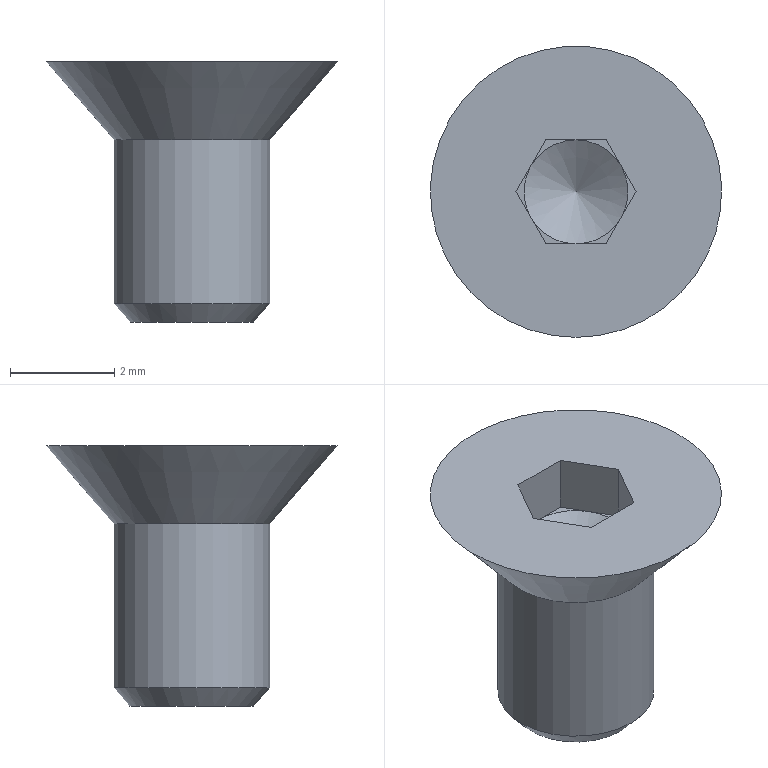Part | NX | features 5003_325_C-SFB3-5 2 | 1 solid | 18 faces | box 5.6 x 5.6 x 5 mm | volume 42.271 mm3 | plane 14 | cone 3 | cylinder 1 | commonest cylinder face diameters 3 x1
STEP:
#1=CARTESIAN_POINT('',(256.67,-34.6,-19.5));
#2=VERTEX_POINT('',#1);
#3=CARTESIAN_POINT('',(257.248,-35.6,-19.5));
#4=VERTEX_POINT('',#3);
#5=CARTESIAN_POINT('',(256.67,-34.6,-19.5));
#6=DIRECTION('',(0.5,-0.866,0.));
#7=VECTOR('',#6,1000.);
#8=LINE('',#5,#7);
#9=EDGE_CURVE('',#2,#4,#8,.T.);
#10=ORIENTED_EDGE('',*,*,#9,.F.);
#11=CARTESIAN_POINT('',(257.248,-33.6,-19.5));
#12=VERTEX_POINT('',#11);
#13=CARTESIAN_POINT('',(257.248,-33.6,-19.5));
#14=DIRECTION('',(-0.5,-0.866,0.));
#15=VECTOR('',#14,1000.);
#16=LINE('',#13,#15);
#17=EDGE_CURVE('',#12,#2,#16,.T.);
#18=ORIENTED_EDGE('',*,*,#17,.F.);
#19=CARTESIAN_POINT('',(258.402,-33.6,-19.5));
#20=VERTEX_POINT('',#19);
#21=CARTESIAN_POINT('',(258.402,-33.6,-19.5));
#22=DIRECTION('',(-1.,0.,0.));
#23=VECTOR('',#22,1000.);
#24=LINE('',#21,#23);
#25=EDGE_CURVE('',#20,#12,#24,.T.);
#26=ORIENTED_EDGE('',*,*,#25,.F.);
#27=CARTESIAN_POINT('',(258.98,-34.6,-19.5));
#28=VERTEX_POINT('',#27);
#29=CARTESIAN_POINT('',(258.98,-34.6,-19.5));
#30=DIRECTION('',(-0.5,0.866,0.));
#31=VECTOR('',#30,1000.);
#32=LINE('',#29,#31);
#33=EDGE_CURVE('',#28,#20,#32,.T.);
#34=ORIENTED_EDGE('',*,*,#33,.F.);
#35=CARTESIAN_POINT('',(258.402,-35.6,-19.5));
#36=VERTEX_POINT('',#35);
#37=CARTESIAN_POINT('',(258.402,-35.6,-19.5));
#38=DIRECTION('',(0.5,0.866,0.));
#39=VECTOR('',#38,1000.);
#40=LINE('',#37,#39);
#41=EDGE_CURVE('',#36,#28,#40,.T.);
#42=ORIENTED_EDGE('',*,*,#41,.F.);
#43=CARTESIAN_POINT('',(257.248,-35.6,-19.5));
#44=DIRECTION('',(1.,0.,0.));
#45=VECTOR('',#44,1000.);
#46=LINE('',#43,#45);
#47=EDGE_CURVE('',#4,#36,#46,.T.);
#48=ORIENTED_EDGE('',*,*,#47,.F.);
#49=EDGE_LOOP('',(#10,#18,#26,#34,#42,#48));
#50=FACE_BOUND('',#49,.T.);
#51=CARTESIAN_POINT('',(257.825,-37.4,-19.5));
#52=VERTEX_POINT('',#51);
#53=CARTESIAN_POINT('',(257.825,-34.6,-19.5));
#54=DIRECTION('',(0.,0.,-1.));
#55=DIRECTION('',(0.,-1.,0.));
#56=AXIS2_PLACEMENT_3D('',#53,#54,#55);
#57=CIRCLE('',#56,2.8);
#58=EDGE_CURVE('',#52,#52,#57,.T.);
#59=ORIENTED_EDGE('',*,*,#58,.F.);
#60=EDGE_LOOP('',(#59));
#61=FACE_BOUND('',#60,.T.);
#62=CARTESIAN_POINT('',(257.825,-34.6,-19.5));
#63=DIRECTION('',(0.,0.,1.));
#64=DIRECTION('',(0.,1.,0.));
#65=AXIS2_PLACEMENT_3D('',#62,#63,#64);
#66=PLANE('',#65);
#67=ADVANCED_FACE('',(#50,#61),#66,.T.);
#68=ORIENTED_EDGE('',*,*,#58,.T.);
#69=EDGE_LOOP('',(#68));
#70=FACE_BOUND('',#69,.T.);
#71=CARTESIAN_POINT('',(257.825,-36.1,-21.));
#72=VERTEX_POINT('',#71);
#73=CARTESIAN_POINT('',(257.825,-34.6,-21.));
#74=DIRECTION('',(0.,0.,-1.));
#75=DIRECTION('',(0.,-1.,0.));
#76=AXIS2_PLACEMENT_3D('',#73,#74,#75);
#77=CIRCLE('',#76,1.5);
#78=EDGE_CURVE('',#72,#72,#77,.T.);
#79=ORIENTED_EDGE('',*,*,#78,.F.);
#80=EDGE_LOOP('',(#79));
#81=FACE_BOUND('',#80,.T.);
#82=CARTESIAN_POINT('',(257.825,-34.6,-21.));
#83=DIRECTION('',(0.,0.,1.));
#84=DIRECTION('',(0.,1.,0.));
#85=AXIS2_PLACEMENT_3D('',#82,#83,#84);
#86=CONICAL_SURFACE('',#85,1.5,0.7141);
#87=ADVANCED_FACE('',(#70,#81),#86,.T.);
#88=ORIENTED_EDGE('',*,*,#78,.T.);
#89=EDGE_LOOP('',(#88));
#90=FACE_BOUND('',#89,.T.);
#91=CARTESIAN_POINT('',(257.825,-36.1,-24.146));
#92=VERTEX_POINT('',#91);
#93=CARTESIAN_POINT('',(257.825,-34.6,-24.146));
#94=DIRECTION('',(0.,0.,-1.));
#95=DIRECTION('',(0.,-1.,0.));
#96=AXIS2_PLACEMENT_3D('',#93,#94,#95);
#97=CIRCLE('',#96,1.5);
#98=EDGE_CURVE('',#92,#92,#97,.T.);
#99=ORIENTED_EDGE('',*,*,#98,.F.);
#100=EDGE_LOOP('',(#99));
#101=FACE_BOUND('',#100,.T.);
#102=CARTESIAN_POINT('',(257.825,-34.6,-24.5));
#103=DIRECTION('',(0.,0.,-1.));
#104=DIRECTION('',(0.,-1.,0.));
#105=AXIS2_PLACEMENT_3D('',#102,#103,#104);
#106=CYLINDRICAL_SURFACE('',#105,1.5);
#107=ADVANCED_FACE('',(#90,#101),#106,.T.);
#108=ORIENTED_EDGE('',*,*,#98,.T.);
#109=EDGE_LOOP('',(#108));
#110=FACE_BOUND('',#109,.T.);
#111=CARTESIAN_POINT('',(257.825,-35.793,-24.5));
#112=VERTEX_POINT('',#111);
#113=CARTESIAN_POINT('',(257.825,-34.6,-24.5));
#114=DIRECTION('',(0.,0.,-1.));
#115=DIRECTION('',(0.,-1.,0.));
#116=AXIS2_PLACEMENT_3D('',#113,#114,#115);
#117=CIRCLE('',#116,1.194);
#118=EDGE_CURVE('',#112,#112,#117,.T.);
#119=ORIENTED_EDGE('',*,*,#118,.F.);
#120=EDGE_LOOP('',(#119));
#121=FACE_BOUND('',#120,.T.);
#122=CARTESIAN_POINT('',(257.825,-34.6,-24.5));
#123=DIRECTION('',(0.,0.,1.));
#124=DIRECTION('',(0.,1.,0.));
#125=AXIS2_PLACEMENT_3D('',#122,#123,#124);
#126=CONICAL_SURFACE('',#125,1.194,0.7141);
#127=ADVANCED_FACE('',(#110,#121),#126,.T.);
#128=ORIENTED_EDGE('',*,*,#118,.T.);
#129=EDGE_LOOP('',(#128));
#130=FACE_BOUND('',#129,.T.);
#131=CARTESIAN_POINT('',(256.632,-34.6,-24.5));
#132=DIRECTION('',(0.,0.,-1.));
#133=DIRECTION('',(0.,-1.,0.));
#134=AXIS2_PLACEMENT_3D('',#131,#132,#133);
#135=PLANE('',#134);
#136=ADVANCED_FACE('',(#130),#135,.T.);
#137=ORIENTED_EDGE('',*,*,#41,.T.);
#138=CARTESIAN_POINT('',(258.98,-34.6,-20.6));
#139=VERTEX_POINT('',#138);
#140=CARTESIAN_POINT('',(258.98,-34.6,-20.6));
#141=DIRECTION('',(0.,0.,1.));
#142=VECTOR('',#141,1000.);
#143=LINE('',#140,#142);
#144=EDGE_CURVE('',#139,#28,#143,.T.);
#145=ORIENTED_EDGE('',*,*,#144,.F.);
#146=CARTESIAN_POINT('',(258.691,-35.1,-20.6));
#147=VERTEX_POINT('',#146);
#148=CARTESIAN_POINT('',(258.402,-35.6,-20.6));
#149=DIRECTION('',(0.5,0.866,0.));
#150=VECTOR('',#149,1000.);
#151=LINE('',#148,#150);
#152=EDGE_CURVE('',#147,#139,#151,.T.);
#153=ORIENTED_EDGE('',*,*,#152,.F.);
#154=CARTESIAN_POINT('',(258.402,-35.6,-20.6));
#155=VERTEX_POINT('',#154);
#156=CARTESIAN_POINT('',(258.402,-35.6,-20.6));
#157=DIRECTION('',(0.5,0.866,0.));
#158=VECTOR('',#157,1000.);
#159=LINE('',#156,#158);
#160=EDGE_CURVE('',#155,#147,#159,.T.);
#161=ORIENTED_EDGE('',*,*,#160,.F.);
#162=CARTESIAN_POINT('',(258.402,-35.6,-20.6));
#163=DIRECTION('',(0.,0.,1.));
#164=VECTOR('',#163,1000.);
#165=LINE('',#162,#164);
#166=EDGE_CURVE('',#155,#36,#165,.T.);
#167=ORIENTED_EDGE('',*,*,#166,.T.);
#168=EDGE_LOOP('',(#137,#145,#153,#161,#167));
#169=FACE_BOUND('',#168,.T.);
#170=CARTESIAN_POINT('',(258.402,-35.6,-20.6));
#171=DIRECTION('',(0.866,-0.5,0.));
#172=DIRECTION('',(-0.5,-0.866,0.));
#173=AXIS2_PLACEMENT_3D('',#170,#171,#172);
#174=PLANE('',#173);
#175=ADVANCED_FACE('',(#169),#174,.F.);
#176=ORIENTED_EDGE('',*,*,#47,.T.);
#177=ORIENTED_EDGE('',*,*,#166,.F.);
#178=CARTESIAN_POINT('',(257.825,-35.6,-20.6));
#179=VERTEX_POINT('',#178);
#180=CARTESIAN_POINT('',(257.248,-35.6,-20.6));
#181=DIRECTION('',(1.,0.,0.));
#182=VECTOR('',#181,1000.);
#183=LINE('',#180,#182);
#184=EDGE_CURVE('',#179,#155,#183,.T.);
#185=ORIENTED_EDGE('',*,*,#184,.F.);
#186=CARTESIAN_POINT('',(257.248,-35.6,-20.6));
#187=VERTEX_POINT('',#186);
#188=CARTESIAN_POINT('',(257.248,-35.6,-20.6));
#189=DIRECTION('',(1.,0.,0.));
#190=VECTOR('',#189,1000.);
#191=LINE('',#188,#190);
#192=EDGE_CURVE('',#187,#179,#191,.T.);
#193=ORIENTED_EDGE('',*,*,#192,.F.);
#194=CARTESIAN_POINT('',(257.248,-35.6,-20.6));
#195=DIRECTION('',(0.,0.,1.));
#196=VECTOR('',#195,1000.);
#197=LINE('',#194,#196);
#198=EDGE_CURVE('',#187,#4,#197,.T.);
#199=ORIENTED_EDGE('',*,*,#198,.T.);
#200=EDGE_LOOP('',(#176,#177,#185,#193,#199));
#201=FACE_BOUND('',#200,.T.);
#202=CARTESIAN_POINT('',(257.248,-35.6,-20.6));
#203=DIRECTION('',(0.,-1.,0.));
#204=DIRECTION('',(-1.,0.,0.));
#205=AXIS2_PLACEMENT_3D('',#202,#203,#204);
#206=PLANE('',#205);
#207=ADVANCED_FACE('',(#201),#206,.F.);
#208=ORIENTED_EDGE('',*,*,#9,.T.);
#209=ORIENTED_EDGE('',*,*,#198,.F.);
#210=CARTESIAN_POINT('',(256.959,-35.1,-20.6));
#211=VERTEX_POINT('',#210);
#212=CARTESIAN_POINT('',(256.67,-34.6,-20.6));
#213=DIRECTION('',(0.5,-0.866,0.));
#214=VECTOR('',#213,1000.);
#215=LINE('',#212,#214);
#216=EDGE_CURVE('',#211,#187,#215,.T.);
#217=ORIENTED_EDGE('',*,*,#216,.F.);
#218=CARTESIAN_POINT('',(256.67,-34.6,-20.6));
#219=VERTEX_POINT('',#218);
#220=CARTESIAN_POINT('',(256.67,-34.6,-20.6));
#221=DIRECTION('',(0.5,-0.866,0.));
#222=VECTOR('',#221,1000.);
#223=LINE('',#220,#222);
#224=EDGE_CURVE('',#219,#211,#223,.T.);
#225=ORIENTED_EDGE('',*,*,#224,.F.);
#226=CARTESIAN_POINT('',(256.67,-34.6,-20.6));
#227=DIRECTION('',(0.,0.,1.));
#228=VECTOR('',#227,1000.);
#229=LINE('',#226,#228);
#230=EDGE_CURVE('',#219,#2,#229,.T.);
#231=ORIENTED_EDGE('',*,*,#230,.T.);
#232=EDGE_LOOP('',(#208,#209,#217,#225,#231));
#233=FACE_BOUND('',#232,.T.);
#234=CARTESIAN_POINT('',(256.67,-34.6,-20.6));
#235=DIRECTION('',(-0.866,-0.5,0.));
#236=DIRECTION('',(-0.5,0.866,0.));
#237=AXIS2_PLACEMENT_3D('',#234,#235,#236);
#238=PLANE('',#237);
#239=ADVANCED_FACE('',(#233),#238,.F.);
#240=ORIENTED_EDGE('',*,*,#17,.T.);
#241=ORIENTED_EDGE('',*,*,#230,.F.);
#242=CARTESIAN_POINT('',(256.959,-34.1,-20.6));
#243=VERTEX_POINT('',#242);
#244=CARTESIAN_POINT('',(257.248,-33.6,-20.6));
#245=DIRECTION('',(-0.5,-0.866,0.));
#246=VECTOR('',#245,1000.);
#247=LINE('',#244,#246);
#248=EDGE_CURVE('',#243,#219,#247,.T.);
#249=ORIENTED_EDGE('',*,*,#248,.F.);
#250=CARTESIAN_POINT('',(257.248,-33.6,-20.6));
#251=VERTEX_POINT('',#250);
#252=CARTESIAN_POINT('',(257.248,-33.6,-20.6));
#253=DIRECTION('',(-0.5,-0.866,0.));
#254=VECTOR('',#253,1000.);
#255=LINE('',#252,#254);
#256=EDGE_CURVE('',#251,#243,#255,.T.);
#257=ORIENTED_EDGE('',*,*,#256,.F.);
#258=CARTESIAN_POINT('',(257.248,-33.6,-20.6));
#259=DIRECTION('',(0.,0.,1.));
#260=VECTOR('',#259,1000.);
#261=LINE('',#258,#260);
#262=EDGE_CURVE('',#251,#12,#261,.T.);
#263=ORIENTED_EDGE('',*,*,#262,.T.);
#264=EDGE_LOOP('',(#240,#241,#249,#257,#263));
#265=FACE_BOUND('',#264,.T.);
#266=CARTESIAN_POINT('',(257.248,-33.6,-20.6));
#267=DIRECTION('',(-0.866,0.5,0.));
#268=DIRECTION('',(0.5,0.866,0.));
#269=AXIS2_PLACEMENT_3D('',#266,#267,#268);
#270=PLANE('',#269);
#271=ADVANCED_FACE('',(#265),#270,.F.);
#272=ORIENTED_EDGE('',*,*,#25,.T.);
#273=ORIENTED_EDGE('',*,*,#262,.F.);
#274=CARTESIAN_POINT('',(257.825,-33.6,-20.6));
#275=VERTEX_POINT('',#274);
#276=CARTESIAN_POINT('',(258.402,-33.6,-20.6));
#277=DIRECTION('',(-1.,0.,0.));
#278=VECTOR('',#277,1000.);
#279=LINE('',#276,#278);
#280=EDGE_CURVE('',#275,#251,#279,.T.);
#281=ORIENTED_EDGE('',*,*,#280,.F.);
#282=CARTESIAN_POINT('',(258.402,-33.6,-20.6));
#283=VERTEX_POINT('',#282);
#284=CARTESIAN_POINT('',(258.402,-33.6,-20.6));
#285=DIRECTION('',(-1.,0.,0.));
#286=VECTOR('',#285,1000.);
#287=LINE('',#284,#286);
#288=EDGE_CURVE('',#283,#275,#287,.T.);
#289=ORIENTED_EDGE('',*,*,#288,.F.);
#290=CARTESIAN_POINT('',(258.402,-33.6,-20.6));
#291=DIRECTION('',(0.,0.,1.));
#292=VECTOR('',#291,1000.);
#293=LINE('',#290,#292);
#294=EDGE_CURVE('',#283,#20,#293,.T.);
#295=ORIENTED_EDGE('',*,*,#294,.T.);
#296=EDGE_LOOP('',(#272,#273,#281,#289,#295));
#297=FACE_BOUND('',#296,.T.);
#298=CARTESIAN_POINT('',(258.402,-33.6,-20.6));
#299=DIRECTION('',(0.,1.,0.));
#300=DIRECTION('',(0.,0.,-1.));
#301=AXIS2_PLACEMENT_3D('',#298,#299,#300);
#302=PLANE('',#301);
#303=ADVANCED_FACE('',(#297),#302,.F.);
#304=ORIENTED_EDGE('',*,*,#33,.T.);
#305=ORIENTED_EDGE('',*,*,#294,.F.);
#306=CARTESIAN_POINT('',(258.691,-34.1,-20.6));
#307=VERTEX_POINT('',#306);
#308=CARTESIAN_POINT('',(258.98,-34.6,-20.6));
#309=DIRECTION('',(-0.5,0.866,0.));
#310=VECTOR('',#309,1000.);
#311=LINE('',#308,#310);
#312=EDGE_CURVE('',#307,#283,#311,.T.);
#313=ORIENTED_EDGE('',*,*,#312,.F.);
#314=CARTESIAN_POINT('',(258.98,-34.6,-20.6));
#315=DIRECTION('',(-0.5,0.866,0.));
#316=VECTOR('',#315,1000.);
#317=LINE('',#314,#316);
#318=EDGE_CURVE('',#139,#307,#317,.T.);
#319=ORIENTED_EDGE('',*,*,#318,.F.);
#320=ORIENTED_EDGE('',*,*,#144,.T.);
#321=EDGE_LOOP('',(#304,#305,#313,#319,#320));
#322=FACE_BOUND('',#321,.T.);
#323=CARTESIAN_POINT('',(258.98,-34.6,-20.6));
#324=DIRECTION('',(0.866,0.5,0.));
#325=DIRECTION('',(0.5,-0.866,0.));
#326=AXIS2_PLACEMENT_3D('',#323,#324,#325);
#327=PLANE('',#326);
#328=ADVANCED_FACE('',(#322),#327,.F.);
#329=CARTESIAN_POINT('',(257.825,-34.6,-20.6));
#330=DIRECTION('',(0.,0.,1.));
#331=DIRECTION('',(0.,1.,0.));
#332=AXIS2_PLACEMENT_3D('',#329,#330,#331);
#333=CIRCLE('',#332,1.);
#334=EDGE_CURVE('',#307,#275,#333,.T.);
#335=ORIENTED_EDGE('',*,*,#334,.F.);
#336=ORIENTED_EDGE('',*,*,#312,.T.);
#337=ORIENTED_EDGE('',*,*,#288,.T.);
#338=EDGE_LOOP('',(#335,#336,#337));
#339=FACE_BOUND('',#338,.T.);
#340=CARTESIAN_POINT('',(257.825,-34.6,-20.6));
#341=DIRECTION('',(0.,0.,1.));
#342=DIRECTION('',(0.,1.,0.));
#343=AXIS2_PLACEMENT_3D('',#340,#341,#342);
#344=PLANE('',#343);
#345=ADVANCED_FACE('',(#339),#344,.T.);
#346=CARTESIAN_POINT('',(257.825,-34.6,-20.6));
#347=DIRECTION('',(0.,0.,1.));
#348=DIRECTION('',(0.,1.,0.));
#349=AXIS2_PLACEMENT_3D('',#346,#347,#348);
#350=CIRCLE('',#349,1.);
#351=EDGE_CURVE('',#147,#307,#350,.T.);
#352=ORIENTED_EDGE('',*,*,#351,.F.);
#353=ORIENTED_EDGE('',*,*,#152,.T.);
#354=ORIENTED_EDGE('',*,*,#318,.T.);
#355=EDGE_LOOP('',(#352,#353,#354));
#356=FACE_BOUND('',#355,.T.);
#357=CARTESIAN_POINT('',(257.825,-34.6,-20.6));
#358=DIRECTION('',(0.,0.,1.));
#359=DIRECTION('',(0.,1.,0.));
#360=AXIS2_PLACEMENT_3D('',#357,#358,#359);
#361=PLANE('',#360);
#362=ADVANCED_FACE('',(#356),#361,.T.);
#363=CARTESIAN_POINT('',(257.825,-34.6,-20.6));
#364=DIRECTION('',(0.,0.,1.));
#365=DIRECTION('',(0.,1.,0.));
#366=AXIS2_PLACEMENT_3D('',#363,#364,#365);
#367=CIRCLE('',#366,1.);
#368=EDGE_CURVE('',#179,#147,#367,.T.);
#369=ORIENTED_EDGE('',*,*,#368,.F.);
#370=ORIENTED_EDGE('',*,*,#184,.T.);
#371=ORIENTED_EDGE('',*,*,#160,.T.);
#372=EDGE_LOOP('',(#369,#370,#371));
#373=FACE_BOUND('',#372,.T.);
#374=CARTESIAN_POINT('',(257.825,-34.6,-20.6));
#375=DIRECTION('',(0.,0.,1.));
#376=DIRECTION('',(0.,1.,0.));
#377=AXIS2_PLACEMENT_3D('',#374,#375,#376);
#378=PLANE('',#377);
#379=ADVANCED_FACE('',(#373),#378,.T.);
#380=CARTESIAN_POINT('',(257.825,-34.6,-20.6));
#381=DIRECTION('',(0.,0.,1.));
#382=DIRECTION('',(0.,1.,0.));
#383=AXIS2_PLACEMENT_3D('',#380,#381,#382);
#384=CIRCLE('',#383,1.);
#385=EDGE_CURVE('',#211,#179,#384,.T.);
#386=ORIENTED_EDGE('',*,*,#385,.F.);
#387=ORIENTED_EDGE('',*,*,#216,.T.);
#388=ORIENTED_EDGE('',*,*,#192,.T.);
#389=EDGE_LOOP('',(#386,#387,#388));
#390=FACE_BOUND('',#389,.T.);
#391=CARTESIAN_POINT('',(257.825,-34.6,-20.6));
#392=DIRECTION('',(0.,0.,1.));
#393=DIRECTION('',(0.,1.,0.));
#394=AXIS2_PLACEMENT_3D('',#391,#392,#393);
#395=PLANE('',#394);
#396=ADVANCED_FACE('',(#390),#395,.T.);
#397=CARTESIAN_POINT('',(257.825,-34.6,-20.6));
#398=DIRECTION('',(0.,0.,1.));
#399=DIRECTION('',(0.,1.,0.));
#400=AXIS2_PLACEMENT_3D('',#397,#398,#399);
#401=CIRCLE('',#400,1.);
#402=EDGE_CURVE('',#243,#211,#401,.T.);
#403=ORIENTED_EDGE('',*,*,#402,.F.);
#404=ORIENTED_EDGE('',*,*,#248,.T.);
#405=ORIENTED_EDGE('',*,*,#224,.T.);
#406=EDGE_LOOP('',(#403,#404,#405));
#407=FACE_BOUND('',#406,.T.);
#408=CARTESIAN_POINT('',(257.825,-34.6,-20.6));
#409=DIRECTION('',(0.,0.,1.));
#410=DIRECTION('',(0.,1.,0.));
#411=AXIS2_PLACEMENT_3D('',#408,#409,#410);
#412=PLANE('',#411);
#413=ADVANCED_FACE('',(#407),#412,.T.);
#414=CARTESIAN_POINT('',(257.825,-34.6,-20.6));
#415=DIRECTION('',(0.,0.,1.));
#416=DIRECTION('',(0.,1.,0.));
#417=AXIS2_PLACEMENT_3D('',#414,#415,#416);
#418=CIRCLE('',#417,1.);
#419=EDGE_CURVE('',#275,#243,#418,.T.);
#420=ORIENTED_EDGE('',*,*,#419,.F.);
#421=ORIENTED_EDGE('',*,*,#280,.T.);
#422=ORIENTED_EDGE('',*,*,#256,.T.);
#423=EDGE_LOOP('',(#420,#421,#422));
#424=FACE_BOUND('',#423,.T.);
#425=CARTESIAN_POINT('',(257.825,-34.6,-20.6));
#426=DIRECTION('',(0.,0.,1.));
#427=DIRECTION('',(0.,1.,0.));
#428=AXIS2_PLACEMENT_3D('',#425,#426,#427);
#429=PLANE('',#428);
#430=ADVANCED_FACE('',(#424),#429,.T.);
#431=CARTESIAN_POINT('',(257.825,-34.6,-21.201));
#432=VERTEX_POINT('',#431);
#433=VERTEX_LOOP('',#432);
#434=FACE_BOUND('',#433,.T.);
#435=ORIENTED_EDGE('',*,*,#419,.T.);
#436=ORIENTED_EDGE('',*,*,#402,.T.);
#437=ORIENTED_EDGE('',*,*,#385,.T.);
#438=ORIENTED_EDGE('',*,*,#368,.T.);
#439=ORIENTED_EDGE('',*,*,#351,.T.);
#440=ORIENTED_EDGE('',*,*,#334,.T.);
#441=EDGE_LOOP('',(#435,#436,#437,#438,#439,#440));
#442=FACE_BOUND('',#441,.T.);
#443=CARTESIAN_POINT('',(257.825,-34.6,-20.6));
#444=DIRECTION('',(0.,0.,1.));
#445=DIRECTION('',(0.,1.,0.));
#446=AXIS2_PLACEMENT_3D('',#443,#444,#445);
#447=CONICAL_SURFACE('',#446,1.,1.03);
#448=ADVANCED_FACE('',(#434,#442),#447,.F.);
#449=CLOSED_SHELL('',(#67,#87,#107,#127,#136,#175,#207,#239,#271,#303,#328,#345,#362,#379,#396,#413,#430,#448));
#450=MANIFOLD_SOLID_BREP('',#449);
#451=(LENGTH_UNIT()NAMED_UNIT(*)SI_UNIT(.MILLI.,.METRE.));
#452=UNCERTAINTY_MEASURE_WITH_UNIT(LENGTH_MEASURE(0.00001),#451,'','');
#453=(NAMED_UNIT(*)PLANE_ANGLE_UNIT()SI_UNIT($,.RADIAN.));
#454=(NAMED_UNIT(*)SI_UNIT($,.STERADIAN.)SOLID_ANGLE_UNIT());
#455=(GEOMETRIC_REPRESENTATION_CONTEXT(3)GLOBAL_UNCERTAINTY_ASSIGNED_CONTEXT((#452))GLOBAL_UNIT_ASSIGNED_CONTEXT((#451,#453,#454))REPRESENTATION_CONTEXT('',''));
#456=ADVANCED_BREP_SHAPE_REPRESENTATION('',(#450),#455);